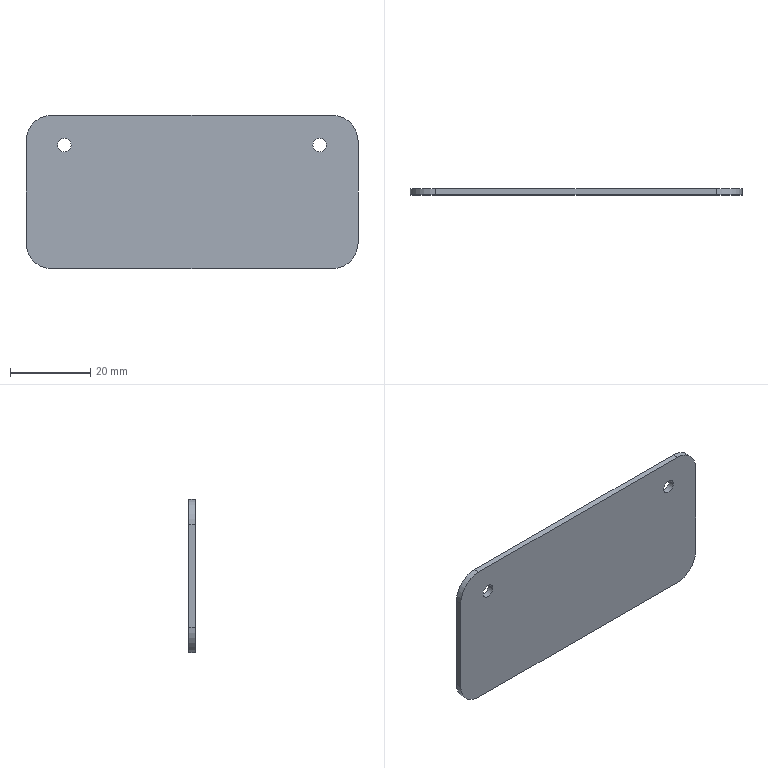Part | NX | features BREP 1 | 1 solid | 14 faces | box 82.55 x 1.499 x 38.1 mm | volume 4635 mm3 | cylinder 8 | plane 6 | commonest cylinder face diameters 3.378 x4 12.7 x4
STEP:
#1=CARTESIAN_POINT('',(-41.275,0.,-12.7));
#2=VERTEX_POINT('',#1);
#3=CARTESIAN_POINT('',(-41.275,0.,12.7));
#4=VERTEX_POINT('',#3);
#5=CARTESIAN_POINT('',(-41.275,0.,-12.7));
#6=DIRECTION('',(0.,0.,1.));
#7=VECTOR('',#6,1000.);
#8=LINE('',#5,#7);
#9=EDGE_CURVE('',#2,#4,#8,.T.);
#10=ORIENTED_EDGE('',*,*,#9,.T.);
#11=CARTESIAN_POINT('',(-34.925,0.,19.05));
#12=VERTEX_POINT('',#11);
#13=CARTESIAN_POINT('',(-34.925,0.,12.7));
#14=DIRECTION('',(0.,1.,0.));
#15=DIRECTION('',(-1.,0.,0.));
#16=AXIS2_PLACEMENT_3D('',#13,#14,#15);
#17=CIRCLE('',#16,6.35);
#18=EDGE_CURVE('',#4,#12,#17,.T.);
#19=ORIENTED_EDGE('',*,*,#18,.T.);
#20=CARTESIAN_POINT('',(34.925,0.,19.05));
#21=VERTEX_POINT('',#20);
#22=CARTESIAN_POINT('',(-34.925,0.,19.05));
#23=DIRECTION('',(1.,0.,0.));
#24=VECTOR('',#23,1000.);
#25=LINE('',#22,#24);
#26=EDGE_CURVE('',#12,#21,#25,.T.);
#27=ORIENTED_EDGE('',*,*,#26,.T.);
#28=CARTESIAN_POINT('',(41.275,0.,12.7));
#29=VERTEX_POINT('',#28);
#30=CARTESIAN_POINT('',(34.925,0.,12.7));
#31=DIRECTION('',(0.,1.,0.));
#32=DIRECTION('',(0.,0.,1.));
#33=AXIS2_PLACEMENT_3D('',#30,#31,#32);
#34=CIRCLE('',#33,6.35);
#35=EDGE_CURVE('',#21,#29,#34,.T.);
#36=ORIENTED_EDGE('',*,*,#35,.T.);
#37=CARTESIAN_POINT('',(41.275,0.,-12.7));
#38=VERTEX_POINT('',#37);
#39=CARTESIAN_POINT('',(41.275,0.,12.7));
#40=DIRECTION('',(0.,0.,-1.));
#41=VECTOR('',#40,1000.);
#42=LINE('',#39,#41);
#43=EDGE_CURVE('',#29,#38,#42,.T.);
#44=ORIENTED_EDGE('',*,*,#43,.T.);
#45=CARTESIAN_POINT('',(34.925,0.,-19.05));
#46=VERTEX_POINT('',#45);
#47=CARTESIAN_POINT('',(34.925,0.,-12.7));
#48=DIRECTION('',(0.,1.,0.));
#49=DIRECTION('',(1.,0.,0.));
#50=AXIS2_PLACEMENT_3D('',#47,#48,#49);
#51=CIRCLE('',#50,6.35);
#52=EDGE_CURVE('',#38,#46,#51,.T.);
#53=ORIENTED_EDGE('',*,*,#52,.T.);
#54=CARTESIAN_POINT('',(-34.925,0.,-19.05));
#55=VERTEX_POINT('',#54);
#56=CARTESIAN_POINT('',(34.925,0.,-19.05));
#57=DIRECTION('',(-1.,0.,0.));
#58=VECTOR('',#57,1000.);
#59=LINE('',#56,#58);
#60=EDGE_CURVE('',#46,#55,#59,.T.);
#61=ORIENTED_EDGE('',*,*,#60,.T.);
#62=CARTESIAN_POINT('',(-34.925,0.,-12.7));
#63=DIRECTION('',(0.,1.,0.));
#64=DIRECTION('',(0.,0.,-1.));
#65=AXIS2_PLACEMENT_3D('',#62,#63,#64);
#66=CIRCLE('',#65,6.35);
#67=EDGE_CURVE('',#55,#2,#66,.T.);
#68=ORIENTED_EDGE('',*,*,#67,.T.);
#69=EDGE_LOOP('',(#10,#19,#27,#36,#44,#53,#61,#68));
#70=FACE_BOUND('',#69,.T.);
#71=CARTESIAN_POINT('',(33.439,0.,11.684));
#72=VERTEX_POINT('',#71);
#73=CARTESIAN_POINT('',(30.061,0.,11.684));
#74=VERTEX_POINT('',#73);
#75=CARTESIAN_POINT('',(31.75,0.,11.684));
#76=DIRECTION('',(0.,1.,0.));
#77=DIRECTION('',(1.,0.,0.));
#78=AXIS2_PLACEMENT_3D('',#75,#76,#77);
#79=CIRCLE('',#78,1.689);
#80=EDGE_CURVE('',#72,#74,#79,.T.);
#81=ORIENTED_EDGE('',*,*,#80,.F.);
#82=CARTESIAN_POINT('',(31.75,0.,11.684));
#83=DIRECTION('',(0.,1.,0.));
#84=DIRECTION('',(-1.,0.,0.));
#85=AXIS2_PLACEMENT_3D('',#82,#83,#84);
#86=CIRCLE('',#85,1.689);
#87=EDGE_CURVE('',#74,#72,#86,.T.);
#88=ORIENTED_EDGE('',*,*,#87,.F.);
#89=EDGE_LOOP('',(#81,#88));
#90=FACE_BOUND('',#89,.T.);
#91=CARTESIAN_POINT('',(-33.439,0.,11.684));
#92=VERTEX_POINT('',#91);
#93=CARTESIAN_POINT('',(-30.061,0.,11.684));
#94=VERTEX_POINT('',#93);
#95=CARTESIAN_POINT('',(-31.75,0.,11.684));
#96=DIRECTION('',(0.,-1.,0.));
#97=DIRECTION('',(-1.,0.,0.));
#98=AXIS2_PLACEMENT_3D('',#95,#96,#97);
#99=CIRCLE('',#98,1.689);
#100=EDGE_CURVE('',#92,#94,#99,.T.);
#101=ORIENTED_EDGE('',*,*,#100,.T.);
#102=CARTESIAN_POINT('',(-31.75,0.,11.684));
#103=DIRECTION('',(0.,-1.,0.));
#104=DIRECTION('',(1.,0.,0.));
#105=AXIS2_PLACEMENT_3D('',#102,#103,#104);
#106=CIRCLE('',#105,1.689);
#107=EDGE_CURVE('',#94,#92,#106,.T.);
#108=ORIENTED_EDGE('',*,*,#107,.T.);
#109=EDGE_LOOP('',(#101,#108));
#110=FACE_BOUND('',#109,.T.);
#111=CARTESIAN_POINT('',(0.,0.,0.));
#112=DIRECTION('',(0.,1.,0.));
#113=DIRECTION('',(1.,0.,0.));
#114=AXIS2_PLACEMENT_3D('',#111,#112,#113);
#115=PLANE('',#114);
#116=ADVANCED_FACE('',(#70,#90,#110),#115,.T.);
#117=CARTESIAN_POINT('',(-34.925,-1.499,-19.05));
#118=VERTEX_POINT('',#117);
#119=CARTESIAN_POINT('',(-34.925,0.,-19.05));
#120=DIRECTION('',(0.,-1.,0.));
#121=VECTOR('',#120,1000.);
#122=LINE('',#119,#121);
#123=EDGE_CURVE('',#55,#118,#122,.T.);
#124=ORIENTED_EDGE('',*,*,#123,.T.);
#125=CARTESIAN_POINT('',(-41.275,-1.499,-12.7));
#126=VERTEX_POINT('',#125);
#127=CARTESIAN_POINT('',(-34.925,-1.499,-12.7));
#128=DIRECTION('',(0.,1.,0.));
#129=DIRECTION('',(0.,0.,-1.));
#130=AXIS2_PLACEMENT_3D('',#127,#128,#129);
#131=CIRCLE('',#130,6.35);
#132=EDGE_CURVE('',#118,#126,#131,.T.);
#133=ORIENTED_EDGE('',*,*,#132,.T.);
#134=CARTESIAN_POINT('',(-41.275,0.,-12.7));
#135=DIRECTION('',(0.,-1.,0.));
#136=VECTOR('',#135,1000.);
#137=LINE('',#134,#136);
#138=EDGE_CURVE('',#2,#126,#137,.T.);
#139=ORIENTED_EDGE('',*,*,#138,.F.);
#140=ORIENTED_EDGE('',*,*,#67,.F.);
#141=EDGE_LOOP('',(#124,#133,#139,#140));
#142=FACE_BOUND('',#141,.T.);
#143=CARTESIAN_POINT('',(-34.925,-0.7493,-12.7));
#144=DIRECTION('',(0.,1.,0.));
#145=DIRECTION('',(0.,0.,-1.));
#146=AXIS2_PLACEMENT_3D('',#143,#144,#145);
#147=CYLINDRICAL_SURFACE('',#146,6.35);
#148=ADVANCED_FACE('',(#142),#147,.T.);
#149=ORIENTED_EDGE('',*,*,#138,.T.);
#150=CARTESIAN_POINT('',(-41.275,-1.499,12.7));
#151=VERTEX_POINT('',#150);
#152=CARTESIAN_POINT('',(-41.275,-1.499,-12.7));
#153=DIRECTION('',(0.,0.,1.));
#154=VECTOR('',#153,1000.);
#155=LINE('',#152,#154);
#156=EDGE_CURVE('',#126,#151,#155,.T.);
#157=ORIENTED_EDGE('',*,*,#156,.T.);
#158=CARTESIAN_POINT('',(-41.275,0.,12.7));
#159=DIRECTION('',(0.,-1.,0.));
#160=VECTOR('',#159,1000.);
#161=LINE('',#158,#160);
#162=EDGE_CURVE('',#4,#151,#161,.T.);
#163=ORIENTED_EDGE('',*,*,#162,.F.);
#164=ORIENTED_EDGE('',*,*,#9,.F.);
#165=EDGE_LOOP('',(#149,#157,#163,#164));
#166=FACE_BOUND('',#165,.T.);
#167=CARTESIAN_POINT('',(-41.275,-0.7493,0.));
#168=DIRECTION('',(-1.,0.,0.));
#169=DIRECTION('',(0.,0.,1.));
#170=AXIS2_PLACEMENT_3D('',#167,#168,#169);
#171=PLANE('',#170);
#172=ADVANCED_FACE('',(#166),#171,.T.);
#173=ORIENTED_EDGE('',*,*,#162,.T.);
#174=CARTESIAN_POINT('',(-34.925,-1.499,19.05));
#175=VERTEX_POINT('',#174);
#176=CARTESIAN_POINT('',(-34.925,-1.499,12.7));
#177=DIRECTION('',(0.,1.,0.));
#178=DIRECTION('',(-1.,0.,0.));
#179=AXIS2_PLACEMENT_3D('',#176,#177,#178);
#180=CIRCLE('',#179,6.35);
#181=EDGE_CURVE('',#151,#175,#180,.T.);
#182=ORIENTED_EDGE('',*,*,#181,.T.);
#183=CARTESIAN_POINT('',(-34.925,0.,19.05));
#184=DIRECTION('',(0.,-1.,0.));
#185=VECTOR('',#184,1000.);
#186=LINE('',#183,#185);
#187=EDGE_CURVE('',#12,#175,#186,.T.);
#188=ORIENTED_EDGE('',*,*,#187,.F.);
#189=ORIENTED_EDGE('',*,*,#18,.F.);
#190=EDGE_LOOP('',(#173,#182,#188,#189));
#191=FACE_BOUND('',#190,.T.);
#192=CARTESIAN_POINT('',(-34.925,-0.7493,12.7));
#193=DIRECTION('',(0.,1.,0.));
#194=DIRECTION('',(-1.,0.,0.));
#195=AXIS2_PLACEMENT_3D('',#192,#193,#194);
#196=CYLINDRICAL_SURFACE('',#195,6.35);
#197=ADVANCED_FACE('',(#191),#196,.T.);
#198=ORIENTED_EDGE('',*,*,#187,.T.);
#199=CARTESIAN_POINT('',(34.925,-1.499,19.05));
#200=VERTEX_POINT('',#199);
#201=CARTESIAN_POINT('',(-34.925,-1.499,19.05));
#202=DIRECTION('',(1.,0.,0.));
#203=VECTOR('',#202,1000.);
#204=LINE('',#201,#203);
#205=EDGE_CURVE('',#175,#200,#204,.T.);
#206=ORIENTED_EDGE('',*,*,#205,.T.);
#207=CARTESIAN_POINT('',(34.925,0.,19.05));
#208=DIRECTION('',(0.,-1.,0.));
#209=VECTOR('',#208,1000.);
#210=LINE('',#207,#209);
#211=EDGE_CURVE('',#21,#200,#210,.T.);
#212=ORIENTED_EDGE('',*,*,#211,.F.);
#213=ORIENTED_EDGE('',*,*,#26,.F.);
#214=EDGE_LOOP('',(#198,#206,#212,#213));
#215=FACE_BOUND('',#214,.T.);
#216=CARTESIAN_POINT('',(0.,-0.7493,19.05));
#217=DIRECTION('',(0.,0.,1.));
#218=DIRECTION('',(1.,0.,0.));
#219=AXIS2_PLACEMENT_3D('',#216,#217,#218);
#220=PLANE('',#219);
#221=ADVANCED_FACE('',(#215),#220,.T.);
#222=ORIENTED_EDGE('',*,*,#211,.T.);
#223=CARTESIAN_POINT('',(41.275,-1.499,12.7));
#224=VERTEX_POINT('',#223);
#225=CARTESIAN_POINT('',(34.925,-1.499,12.7));
#226=DIRECTION('',(0.,1.,0.));
#227=DIRECTION('',(0.,0.,1.));
#228=AXIS2_PLACEMENT_3D('',#225,#226,#227);
#229=CIRCLE('',#228,6.35);
#230=EDGE_CURVE('',#200,#224,#229,.T.);
#231=ORIENTED_EDGE('',*,*,#230,.T.);
#232=CARTESIAN_POINT('',(41.275,0.,12.7));
#233=DIRECTION('',(0.,-1.,0.));
#234=VECTOR('',#233,1000.);
#235=LINE('',#232,#234);
#236=EDGE_CURVE('',#29,#224,#235,.T.);
#237=ORIENTED_EDGE('',*,*,#236,.F.);
#238=ORIENTED_EDGE('',*,*,#35,.F.);
#239=EDGE_LOOP('',(#222,#231,#237,#238));
#240=FACE_BOUND('',#239,.T.);
#241=CARTESIAN_POINT('',(34.925,-0.7493,12.7));
#242=DIRECTION('',(0.,1.,0.));
#243=DIRECTION('',(0.,0.,1.));
#244=AXIS2_PLACEMENT_3D('',#241,#242,#243);
#245=CYLINDRICAL_SURFACE('',#244,6.35);
#246=ADVANCED_FACE('',(#240),#245,.T.);
#247=ORIENTED_EDGE('',*,*,#236,.T.);
#248=CARTESIAN_POINT('',(41.275,-1.499,-12.7));
#249=VERTEX_POINT('',#248);
#250=CARTESIAN_POINT('',(41.275,-1.499,12.7));
#251=DIRECTION('',(0.,0.,-1.));
#252=VECTOR('',#251,1000.);
#253=LINE('',#250,#252);
#254=EDGE_CURVE('',#224,#249,#253,.T.);
#255=ORIENTED_EDGE('',*,*,#254,.T.);
#256=CARTESIAN_POINT('',(41.275,0.,-12.7));
#257=DIRECTION('',(0.,-1.,0.));
#258=VECTOR('',#257,1000.);
#259=LINE('',#256,#258);
#260=EDGE_CURVE('',#38,#249,#259,.T.);
#261=ORIENTED_EDGE('',*,*,#260,.F.);
#262=ORIENTED_EDGE('',*,*,#43,.F.);
#263=EDGE_LOOP('',(#247,#255,#261,#262));
#264=FACE_BOUND('',#263,.T.);
#265=CARTESIAN_POINT('',(41.275,-0.7493,0.));
#266=DIRECTION('',(1.,0.,0.));
#267=DIRECTION('',(0.,1.,0.));
#268=AXIS2_PLACEMENT_3D('',#265,#266,#267);
#269=PLANE('',#268);
#270=ADVANCED_FACE('',(#264),#269,.T.);
#271=ORIENTED_EDGE('',*,*,#260,.T.);
#272=CARTESIAN_POINT('',(34.925,-1.499,-19.05));
#273=VERTEX_POINT('',#272);
#274=CARTESIAN_POINT('',(34.925,-1.499,-12.7));
#275=DIRECTION('',(0.,1.,0.));
#276=DIRECTION('',(1.,0.,0.));
#277=AXIS2_PLACEMENT_3D('',#274,#275,#276);
#278=CIRCLE('',#277,6.35);
#279=EDGE_CURVE('',#249,#273,#278,.T.);
#280=ORIENTED_EDGE('',*,*,#279,.T.);
#281=CARTESIAN_POINT('',(34.925,0.,-19.05));
#282=DIRECTION('',(0.,-1.,0.));
#283=VECTOR('',#282,1000.);
#284=LINE('',#281,#283);
#285=EDGE_CURVE('',#46,#273,#284,.T.);
#286=ORIENTED_EDGE('',*,*,#285,.F.);
#287=ORIENTED_EDGE('',*,*,#52,.F.);
#288=EDGE_LOOP('',(#271,#280,#286,#287));
#289=FACE_BOUND('',#288,.T.);
#290=CARTESIAN_POINT('',(34.925,-0.7493,-12.7));
#291=DIRECTION('',(0.,1.,0.));
#292=DIRECTION('',(1.,0.,0.));
#293=AXIS2_PLACEMENT_3D('',#290,#291,#292);
#294=CYLINDRICAL_SURFACE('',#293,6.35);
#295=ADVANCED_FACE('',(#289),#294,.T.);
#296=ORIENTED_EDGE('',*,*,#285,.T.);
#297=CARTESIAN_POINT('',(34.925,-1.499,-19.05));
#298=DIRECTION('',(-1.,0.,0.));
#299=VECTOR('',#298,1000.);
#300=LINE('',#297,#299);
#301=EDGE_CURVE('',#273,#118,#300,.T.);
#302=ORIENTED_EDGE('',*,*,#301,.T.);
#303=ORIENTED_EDGE('',*,*,#123,.F.);
#304=ORIENTED_EDGE('',*,*,#60,.F.);
#305=EDGE_LOOP('',(#296,#302,#303,#304));
#306=FACE_BOUND('',#305,.T.);
#307=CARTESIAN_POINT('',(0.,-0.7493,-19.05));
#308=DIRECTION('',(0.,0.,-1.));
#309=DIRECTION('',(0.,-1.,0.));
#310=AXIS2_PLACEMENT_3D('',#307,#308,#309);
#311=PLANE('',#310);
#312=ADVANCED_FACE('',(#306),#311,.T.);
#313=ORIENTED_EDGE('',*,*,#301,.F.);
#314=ORIENTED_EDGE('',*,*,#279,.F.);
#315=ORIENTED_EDGE('',*,*,#254,.F.);
#316=ORIENTED_EDGE('',*,*,#230,.F.);
#317=ORIENTED_EDGE('',*,*,#205,.F.);
#318=ORIENTED_EDGE('',*,*,#181,.F.);
#319=ORIENTED_EDGE('',*,*,#156,.F.);
#320=ORIENTED_EDGE('',*,*,#132,.F.);
#321=EDGE_LOOP('',(#313,#314,#315,#316,#317,#318,#319,#320));
#322=FACE_BOUND('',#321,.T.);
#323=CARTESIAN_POINT('',(33.439,-1.499,11.684));
#324=VERTEX_POINT('',#323);
#325=CARTESIAN_POINT('',(30.061,-1.499,11.684));
#326=VERTEX_POINT('',#325);
#327=CARTESIAN_POINT('',(31.75,-1.499,11.684));
#328=DIRECTION('',(0.,1.,0.));
#329=DIRECTION('',(1.,0.,0.));
#330=AXIS2_PLACEMENT_3D('',#327,#328,#329);
#331=CIRCLE('',#330,1.689);
#332=EDGE_CURVE('',#324,#326,#331,.T.);
#333=ORIENTED_EDGE('',*,*,#332,.T.);
#334=CARTESIAN_POINT('',(31.75,-1.499,11.684));
#335=DIRECTION('',(0.,1.,0.));
#336=DIRECTION('',(-1.,0.,0.));
#337=AXIS2_PLACEMENT_3D('',#334,#335,#336);
#338=CIRCLE('',#337,1.689);
#339=EDGE_CURVE('',#326,#324,#338,.T.);
#340=ORIENTED_EDGE('',*,*,#339,.T.);
#341=EDGE_LOOP('',(#333,#340));
#342=FACE_BOUND('',#341,.T.);
#343=CARTESIAN_POINT('',(-33.439,-1.499,11.684));
#344=VERTEX_POINT('',#343);
#345=CARTESIAN_POINT('',(-30.061,-1.499,11.684));
#346=VERTEX_POINT('',#345);
#347=CARTESIAN_POINT('',(-31.75,-1.499,11.684));
#348=DIRECTION('',(0.,-1.,0.));
#349=DIRECTION('',(-1.,0.,0.));
#350=AXIS2_PLACEMENT_3D('',#347,#348,#349);
#351=CIRCLE('',#350,1.689);
#352=EDGE_CURVE('',#344,#346,#351,.T.);
#353=ORIENTED_EDGE('',*,*,#352,.F.);
#354=CARTESIAN_POINT('',(-31.75,-1.499,11.684));
#355=DIRECTION('',(0.,-1.,0.));
#356=DIRECTION('',(1.,0.,0.));
#357=AXIS2_PLACEMENT_3D('',#354,#355,#356);
#358=CIRCLE('',#357,1.689);
#359=EDGE_CURVE('',#346,#344,#358,.T.);
#360=ORIENTED_EDGE('',*,*,#359,.F.);
#361=EDGE_LOOP('',(#353,#360));
#362=FACE_BOUND('',#361,.T.);
#363=CARTESIAN_POINT('',(0.,-1.499,0.));
#364=DIRECTION('',(0.,1.,0.));
#365=DIRECTION('',(1.,0.,0.));
#366=AXIS2_PLACEMENT_3D('',#363,#364,#365);
#367=PLANE('',#366);
#368=ADVANCED_FACE('',(#322,#342,#362),#367,.F.);
#369=CARTESIAN_POINT('',(33.439,0.,11.684));
#370=DIRECTION('',(0.,-1.,0.));
#371=VECTOR('',#370,1000.);
#372=LINE('',#369,#371);
#373=EDGE_CURVE('',#324,#72,#372,.F.);
#374=ORIENTED_EDGE('',*,*,#373,.F.);
#375=ORIENTED_EDGE('',*,*,#339,.F.);
#376=CARTESIAN_POINT('',(30.061,0.,11.684));
#377=DIRECTION('',(0.,-1.,0.));
#378=VECTOR('',#377,1000.);
#379=LINE('',#376,#378);
#380=EDGE_CURVE('',#326,#74,#379,.F.);
#381=ORIENTED_EDGE('',*,*,#380,.T.);
#382=ORIENTED_EDGE('',*,*,#87,.T.);
#383=EDGE_LOOP('',(#374,#375,#381,#382));
#384=FACE_BOUND('',#383,.T.);
#385=CARTESIAN_POINT('',(31.75,-0.7493,11.684));
#386=DIRECTION('',(0.,1.,0.));
#387=DIRECTION('',(-1.,0.,0.));
#388=AXIS2_PLACEMENT_3D('',#385,#386,#387);
#389=CYLINDRICAL_SURFACE('',#388,1.689);
#390=ADVANCED_FACE('',(#384),#389,.F.);
#391=ORIENTED_EDGE('',*,*,#380,.F.);
#392=ORIENTED_EDGE('',*,*,#332,.F.);
#393=ORIENTED_EDGE('',*,*,#373,.T.);
#394=ORIENTED_EDGE('',*,*,#80,.T.);
#395=EDGE_LOOP('',(#391,#392,#393,#394));
#396=FACE_BOUND('',#395,.T.);
#397=CARTESIAN_POINT('',(31.75,-0.7493,11.684));
#398=DIRECTION('',(0.,1.,0.));
#399=DIRECTION('',(1.,0.,0.));
#400=AXIS2_PLACEMENT_3D('',#397,#398,#399);
#401=CYLINDRICAL_SURFACE('',#400,1.689);
#402=ADVANCED_FACE('',(#396),#401,.F.);
#403=CARTESIAN_POINT('',(-30.061,0.,11.684));
#404=DIRECTION('',(0.,-1.,0.));
#405=VECTOR('',#404,1000.);
#406=LINE('',#403,#405);
#407=EDGE_CURVE('',#346,#94,#406,.F.);
#408=ORIENTED_EDGE('',*,*,#407,.F.);
#409=ORIENTED_EDGE('',*,*,#359,.T.);
#410=CARTESIAN_POINT('',(-33.439,0.,11.684));
#411=DIRECTION('',(0.,-1.,0.));
#412=VECTOR('',#411,1000.);
#413=LINE('',#410,#412);
#414=EDGE_CURVE('',#344,#92,#413,.F.);
#415=ORIENTED_EDGE('',*,*,#414,.T.);
#416=ORIENTED_EDGE('',*,*,#107,.F.);
#417=EDGE_LOOP('',(#408,#409,#415,#416));
#418=FACE_BOUND('',#417,.T.);
#419=CARTESIAN_POINT('',(-31.75,-0.7493,11.684));
#420=DIRECTION('',(0.,-1.,0.));
#421=DIRECTION('',(1.,0.,0.));
#422=AXIS2_PLACEMENT_3D('',#419,#420,#421);
#423=CYLINDRICAL_SURFACE('',#422,1.689);
#424=ADVANCED_FACE('',(#418),#423,.F.);
#425=ORIENTED_EDGE('',*,*,#414,.F.);
#426=ORIENTED_EDGE('',*,*,#352,.T.);
#427=ORIENTED_EDGE('',*,*,#407,.T.);
#428=ORIENTED_EDGE('',*,*,#100,.F.);
#429=EDGE_LOOP('',(#425,#426,#427,#428));
#430=FACE_BOUND('',#429,.T.);
#431=CARTESIAN_POINT('',(-31.75,-0.7493,11.684));
#432=DIRECTION('',(0.,-1.,0.));
#433=DIRECTION('',(-1.,0.,0.));
#434=AXIS2_PLACEMENT_3D('',#431,#432,#433);
#435=CYLINDRICAL_SURFACE('',#434,1.689);
#436=ADVANCED_FACE('',(#430),#435,.F.);
#437=CLOSED_SHELL('',(#116,#148,#172,#197,#221,#246,#270,#295,#312,#368,#390,#402,#424,#436));
#438=MANIFOLD_SOLID_BREP('',#437);
#439=(LENGTH_UNIT()NAMED_UNIT(*)SI_UNIT(.MILLI.,.METRE.));
#440=UNCERTAINTY_MEASURE_WITH_UNIT(LENGTH_MEASURE(0.00001),#439,'','');
#441=(NAMED_UNIT(*)PLANE_ANGLE_UNIT()SI_UNIT($,.RADIAN.));
#442=(NAMED_UNIT(*)SI_UNIT($,.STERADIAN.)SOLID_ANGLE_UNIT());
#443=(GEOMETRIC_REPRESENTATION_CONTEXT(3)GLOBAL_UNCERTAINTY_ASSIGNED_CONTEXT((#440))GLOBAL_UNIT_ASSIGNED_CONTEXT((#439,#441,#442))REPRESENTATION_CONTEXT('',''));
#444=ADVANCED_BREP_SHAPE_REPRESENTATION('',(#438),#443);